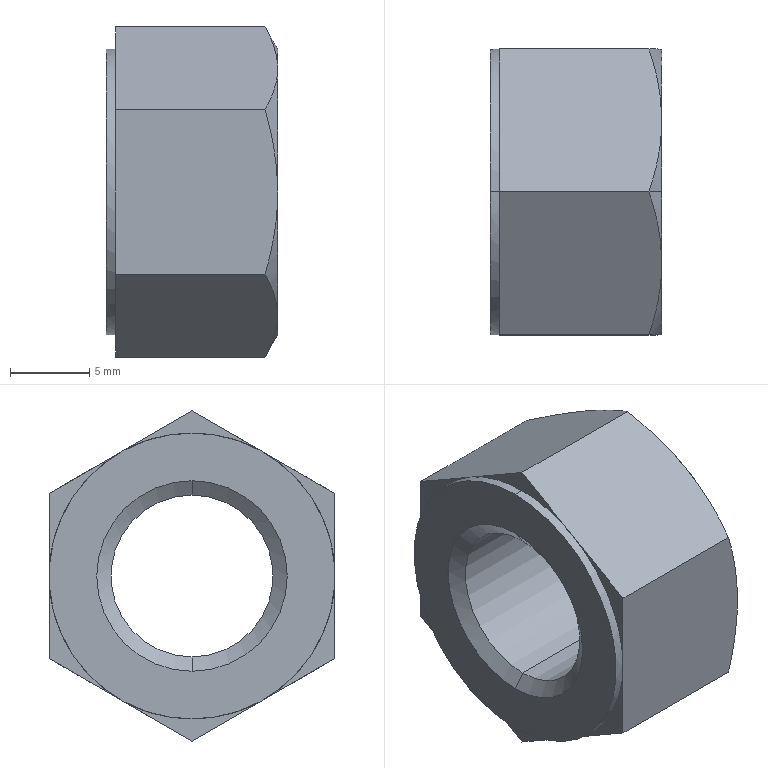Part | SolidWorks | features BaseBody 1 | 1 solid | 31 faces | box 10.8 x 18 x 20.785 mm | volume 2106 mm3 | plane 14 | cone 11 | cylinder 6 | commonest cylinder face diameters 10.2 x2 12 x2 18 x2
STEP:
#1=CARTESIAN_POINT('',(235.656,-84.,194.721));
#2=VERTEX_POINT('',#1);
#3=CARTESIAN_POINT('',(235.656,-84.,184.521));
#4=VERTEX_POINT('',#3);
#5=CARTESIAN_POINT('',(235.656,-84.,189.621));
#6=DIRECTION('',(1.,0.,0.));
#7=DIRECTION('',(0.,0.,-1.));
#8=AXIS2_PLACEMENT_3D('',#5,#6,#7);
#9=CIRCLE('',#8,5.1);
#10=EDGE_CURVE('',#2,#4,#9,.T.);
#11=ORIENTED_EDGE('',*,*,#10,.F.);
#12=CARTESIAN_POINT('',(245.17,-84.,194.721));
#13=VERTEX_POINT('',#12);
#14=CARTESIAN_POINT('',(235.,-84.,194.721));
#15=DIRECTION('',(1.,0.,0.));
#16=VECTOR('',#15,1000.);
#17=LINE('',#14,#16);
#18=EDGE_CURVE('',#2,#13,#17,.T.);
#19=ORIENTED_EDGE('',*,*,#18,.T.);
#20=CARTESIAN_POINT('',(245.17,-84.,184.521));
#21=VERTEX_POINT('',#20);
#22=CARTESIAN_POINT('',(245.17,-84.,189.621));
#23=DIRECTION('',(-1.,0.,0.));
#24=DIRECTION('',(0.,0.,-1.));
#25=AXIS2_PLACEMENT_3D('',#22,#23,#24);
#26=CIRCLE('',#25,5.1);
#27=EDGE_CURVE('',#21,#13,#26,.T.);
#28=ORIENTED_EDGE('',*,*,#27,.F.);
#29=CARTESIAN_POINT('',(235.,-84.,184.521));
#30=DIRECTION('',(1.,0.,0.));
#31=VECTOR('',#30,1000.);
#32=LINE('',#29,#31);
#33=EDGE_CURVE('',#4,#21,#32,.T.);
#34=ORIENTED_EDGE('',*,*,#33,.F.);
#35=EDGE_LOOP('',(#11,#19,#28,#34));
#36=FACE_OUTER_BOUND('',#35,.T.);
#37=CARTESIAN_POINT('',(235.,-84.,189.621));
#38=DIRECTION('',(1.,0.,0.));
#39=DIRECTION('',(0.,0.,-1.));
#40=AXIS2_PLACEMENT_3D('',#37,#38,#39);
#41=CYLINDRICAL_SURFACE('',#40,5.1);
#42=ADVANCED_FACE('',(#36),#41,.F.);
#43=ORIENTED_EDGE('',*,*,#27,.T.);
#44=CARTESIAN_POINT('',(245.8,-84.,195.621));
#45=VERTEX_POINT('',#44);
#46=CARTESIAN_POINT('',(245.8,-84.,195.621));
#47=DIRECTION('',(0.5736,0.,0.8192));
#48=VECTOR('',#47,1000.);
#49=LINE('',#46,#48);
#50=EDGE_CURVE('',#13,#45,#49,.T.);
#51=ORIENTED_EDGE('',*,*,#50,.T.);
#52=CARTESIAN_POINT('',(245.8,-84.,183.621));
#53=VERTEX_POINT('',#52);
#54=CARTESIAN_POINT('',(245.8,-84.,189.621));
#55=DIRECTION('',(-1.,0.,0.));
#56=DIRECTION('',(0.,0.,-1.));
#57=AXIS2_PLACEMENT_3D('',#54,#55,#56);
#58=CIRCLE('',#57,6.);
#59=EDGE_CURVE('',#53,#45,#58,.T.);
#60=ORIENTED_EDGE('',*,*,#59,.F.);
#61=CARTESIAN_POINT('',(245.8,-84.,183.621));
#62=DIRECTION('',(0.5736,0.,-0.8192));
#63=VECTOR('',#62,1000.);
#64=LINE('',#61,#63);
#65=EDGE_CURVE('',#21,#53,#64,.T.);
#66=ORIENTED_EDGE('',*,*,#65,.F.);
#67=EDGE_LOOP('',(#43,#51,#60,#66));
#68=FACE_OUTER_BOUND('',#67,.T.);
#69=CARTESIAN_POINT('',(245.8,-84.,189.621));
#70=DIRECTION('',(1.,0.,0.));
#71=DIRECTION('',(0.,0.,-1.));
#72=AXIS2_PLACEMENT_3D('',#69,#70,#71);
#73=CONICAL_SURFACE('',#72,6.,0.9599);
#74=ADVANCED_FACE('',(#68),#73,.F.);
#75=ORIENTED_EDGE('',*,*,#10,.T.);
#76=CARTESIAN_POINT('',(235.025,-84.,183.621));
#77=VERTEX_POINT('',#76);
#78=CARTESIAN_POINT('',(235.025,-84.,183.621));
#79=DIRECTION('',(-0.5736,0.,-0.8192));
#80=VECTOR('',#79,1000.);
#81=LINE('',#78,#80);
#82=EDGE_CURVE('',#4,#77,#81,.T.);
#83=ORIENTED_EDGE('',*,*,#82,.T.);
#84=CARTESIAN_POINT('',(235.025,-84.,195.621));
#85=VERTEX_POINT('',#84);
#86=CARTESIAN_POINT('',(235.025,-84.,189.621));
#87=DIRECTION('',(1.,0.,0.));
#88=DIRECTION('',(0.,-0.5,-0.866));
#89=AXIS2_PLACEMENT_3D('',#86,#87,#88);
#90=CIRCLE('',#89,6.);
#91=EDGE_CURVE('',#85,#77,#90,.T.);
#92=ORIENTED_EDGE('',*,*,#91,.F.);
#93=CARTESIAN_POINT('',(235.025,-84.,195.621));
#94=DIRECTION('',(-0.5736,0.,0.8192));
#95=VECTOR('',#94,1000.);
#96=LINE('',#93,#95);
#97=EDGE_CURVE('',#2,#85,#96,.T.);
#98=ORIENTED_EDGE('',*,*,#97,.F.);
#99=EDGE_LOOP('',(#75,#83,#92,#98));
#100=FACE_OUTER_BOUND('',#99,.T.);
#101=CARTESIAN_POINT('',(235.025,-84.,189.621));
#102=DIRECTION('',(-1.,0.,0.));
#103=DIRECTION('',(0.,0.,1.));
#104=AXIS2_PLACEMENT_3D('',#101,#102,#103);
#105=CONICAL_SURFACE('',#104,6.,0.9599);
#106=ADVANCED_FACE('',(#100),#105,.F.);
#107=CARTESIAN_POINT('',(235.,-84.,195.621));
#108=VERTEX_POINT('',#107);
#109=CARTESIAN_POINT('',(235.,-84.,183.621));
#110=VERTEX_POINT('',#109);
#111=CARTESIAN_POINT('',(235.,-84.,189.621));
#112=DIRECTION('',(1.,0.,0.));
#113=DIRECTION('',(0.,0.,-1.));
#114=AXIS2_PLACEMENT_3D('',#111,#112,#113);
#115=CIRCLE('',#114,6.);
#116=EDGE_CURVE('',#108,#110,#115,.T.);
#117=ORIENTED_EDGE('',*,*,#116,.F.);
#118=CARTESIAN_POINT('',(220.762,-84.,195.621));
#119=DIRECTION('',(1.,0.,0.));
#120=VECTOR('',#119,1000.);
#121=LINE('',#118,#120);
#122=EDGE_CURVE('',#108,#85,#121,.T.);
#123=ORIENTED_EDGE('',*,*,#122,.T.);
#124=ORIENTED_EDGE('',*,*,#91,.T.);
#125=CARTESIAN_POINT('',(220.762,-84.,183.621));
#126=DIRECTION('',(1.,0.,0.));
#127=VECTOR('',#126,1000.);
#128=LINE('',#125,#127);
#129=EDGE_CURVE('',#110,#77,#128,.T.);
#130=ORIENTED_EDGE('',*,*,#129,.F.);
#131=EDGE_LOOP('',(#117,#123,#124,#130));
#132=FACE_OUTER_BOUND('',#131,.T.);
#133=CARTESIAN_POINT('',(220.762,-84.,189.621));
#134=DIRECTION('',(1.,0.,0.));
#135=DIRECTION('',(0.,0.,-1.));
#136=AXIS2_PLACEMENT_3D('',#133,#134,#135);
#137=CYLINDRICAL_SURFACE('',#136,6.);
#138=ADVANCED_FACE('',(#132),#137,.F.);
#139=CARTESIAN_POINT('',(245.8,-88.5,197.415));
#140=VERTEX_POINT('',#139);
#141=CARTESIAN_POINT('',(245.8,-84.,198.621));
#142=VERTEX_POINT('',#141);
#143=CARTESIAN_POINT('',(245.8,-84.,189.621));
#144=DIRECTION('',(-1.,0.,0.));
#145=DIRECTION('',(0.,0.,1.));
#146=AXIS2_PLACEMENT_3D('',#143,#144,#145);
#147=CIRCLE('',#146,9.);
#148=EDGE_CURVE('',#140,#142,#147,.T.);
#149=ORIENTED_EDGE('',*,*,#148,.T.);
#150=CARTESIAN_POINT('',(244.996,-84.,200.013));
#151=VERTEX_POINT('',#150);
#152=CARTESIAN_POINT('',(244.991,-84.,200.022));
#153=DIRECTION('',(-0.5,0.,0.866));
#154=VECTOR('',#153,1000.);
#155=LINE('',#152,#154);
#156=EDGE_CURVE('',#142,#151,#155,.T.);
#157=ORIENTED_EDGE('',*,*,#156,.T.);
#158=CARTESIAN_POINT('',(244.996,-84.,200.013));
#159=CARTESIAN_POINT('',(245.241,-84.735,199.589));
#160=CARTESIAN_POINT('',(245.443,-85.476,199.161));
#161=CARTESIAN_POINT('',(245.723,-86.974,198.296));
#162=CARTESIAN_POINT('',(245.8,-87.732,197.859));
#163=CARTESIAN_POINT('',(245.8,-88.5,197.415));
#164=B_SPLINE_CURVE_WITH_KNOTS('',3,(#158,#159,#160,#161,#162,#163),.UNSPECIFIED.,.F.,.F.,(4,2,4),(0.,0.002629,0.005258),.UNSPECIFIED.);
#165=EDGE_CURVE('',#151,#140,#164,.T.);
#166=ORIENTED_EDGE('',*,*,#165,.T.);
#167=EDGE_LOOP('',(#149,#157,#166));
#168=FACE_OUTER_BOUND('',#167,.T.);
#169=CARTESIAN_POINT('',(244.991,-84.,189.621));
#170=DIRECTION('',(-1.,0.,0.));
#171=DIRECTION('',(0.,0.,1.));
#172=AXIS2_PLACEMENT_3D('',#169,#170,#171);
#173=CONICAL_SURFACE('',#172,10.401,1.047);
#174=ADVANCED_FACE('',(#168),#173,.T.);
#175=CARTESIAN_POINT('',(235.,-84.,198.621));
#176=VERTEX_POINT('',#175);
#177=CARTESIAN_POINT('',(235.,-84.,180.621));
#178=VERTEX_POINT('',#177);
#179=CARTESIAN_POINT('',(235.,-84.,189.621));
#180=DIRECTION('',(-1.,0.,0.));
#181=DIRECTION('',(0.,0.,-1.));
#182=AXIS2_PLACEMENT_3D('',#179,#180,#181);
#183=CIRCLE('',#182,9.);
#184=EDGE_CURVE('',#176,#178,#183,.T.);
#185=ORIENTED_EDGE('',*,*,#184,.F.);
#186=CARTESIAN_POINT('',(235.6,-84.,198.621));
#187=VERTEX_POINT('',#186);
#188=CARTESIAN_POINT('',(245.8,-84.,198.621));
#189=DIRECTION('',(1.,0.,0.));
#190=VECTOR('',#189,1000.);
#191=LINE('',#188,#190);
#192=EDGE_CURVE('',#176,#187,#191,.T.);
#193=ORIENTED_EDGE('',*,*,#192,.T.);
#194=CARTESIAN_POINT('',(235.6,-79.5,197.415));
#195=VERTEX_POINT('',#194);
#196=CARTESIAN_POINT('',(235.6,-84.,189.621));
#197=DIRECTION('',(-1.,0.,0.));
#198=DIRECTION('',(0.,0.,-1.));
#199=AXIS2_PLACEMENT_3D('',#196,#197,#198);
#200=CIRCLE('',#199,9.);
#201=EDGE_CURVE('',#187,#195,#200,.T.);
#202=ORIENTED_EDGE('',*,*,#201,.T.);
#203=CARTESIAN_POINT('',(235.6,-75.,189.621));
#204=VERTEX_POINT('',#203);
#205=CARTESIAN_POINT('',(235.6,-84.,189.621));
#206=DIRECTION('',(-1.,0.,0.));
#207=DIRECTION('',(0.,0.,-1.));
#208=AXIS2_PLACEMENT_3D('',#205,#206,#207);
#209=CIRCLE('',#208,9.);
#210=EDGE_CURVE('',#195,#204,#209,.T.);
#211=ORIENTED_EDGE('',*,*,#210,.T.);
#212=CARTESIAN_POINT('',(235.6,-79.5,181.827));
#213=VERTEX_POINT('',#212);
#214=CARTESIAN_POINT('',(235.6,-84.,189.621));
#215=DIRECTION('',(-1.,0.,0.));
#216=DIRECTION('',(0.,0.,-1.));
#217=AXIS2_PLACEMENT_3D('',#214,#215,#216);
#218=CIRCLE('',#217,9.);
#219=EDGE_CURVE('',#204,#213,#218,.T.);
#220=ORIENTED_EDGE('',*,*,#219,.T.);
#221=CARTESIAN_POINT('',(235.6,-84.,180.621));
#222=VERTEX_POINT('',#221);
#223=CARTESIAN_POINT('',(235.6,-84.,189.621));
#224=DIRECTION('',(-1.,0.,0.));
#225=DIRECTION('',(0.,0.,-1.));
#226=AXIS2_PLACEMENT_3D('',#223,#224,#225);
#227=CIRCLE('',#226,9.);
#228=EDGE_CURVE('',#213,#222,#227,.T.);
#229=ORIENTED_EDGE('',*,*,#228,.T.);
#230=CARTESIAN_POINT('',(245.8,-84.,180.621));
#231=DIRECTION('',(1.,0.,0.));
#232=VECTOR('',#231,1000.);
#233=LINE('',#230,#232);
#234=EDGE_CURVE('',#178,#222,#233,.T.);
#235=ORIENTED_EDGE('',*,*,#234,.F.);
#236=EDGE_LOOP('',(#185,#193,#202,#211,#220,#229,#235));
#237=FACE_OUTER_BOUND('',#236,.T.);
#238=CARTESIAN_POINT('',(245.8,-84.,189.621));
#239=DIRECTION('',(1.,0.,0.));
#240=DIRECTION('',(0.,0.,-1.));
#241=AXIS2_PLACEMENT_3D('',#238,#239,#240);
#242=CYLINDRICAL_SURFACE('',#241,9.);
#243=ADVANCED_FACE('',(#237),#242,.T.);
#244=ORIENTED_EDGE('',*,*,#18,.F.);
#245=CARTESIAN_POINT('',(235.656,-84.,189.621));
#246=DIRECTION('',(1.,0.,0.));
#247=DIRECTION('',(0.,0.,-1.));
#248=AXIS2_PLACEMENT_3D('',#245,#246,#247);
#249=CIRCLE('',#248,5.1);
#250=EDGE_CURVE('',#4,#2,#249,.T.);
#251=ORIENTED_EDGE('',*,*,#250,.F.);
#252=ORIENTED_EDGE('',*,*,#33,.T.);
#253=CARTESIAN_POINT('',(245.17,-84.,189.621));
#254=DIRECTION('',(-1.,0.,0.));
#255=DIRECTION('',(0.,0.,-1.));
#256=AXIS2_PLACEMENT_3D('',#253,#254,#255);
#257=CIRCLE('',#256,5.1);
#258=EDGE_CURVE('',#13,#21,#257,.T.);
#259=ORIENTED_EDGE('',*,*,#258,.F.);
#260=EDGE_LOOP('',(#244,#251,#252,#259));
#261=FACE_OUTER_BOUND('',#260,.T.);
#262=CARTESIAN_POINT('',(235.,-84.,189.621));
#263=DIRECTION('',(1.,0.,0.));
#264=DIRECTION('',(0.,0.,-1.));
#265=AXIS2_PLACEMENT_3D('',#262,#263,#264);
#266=CYLINDRICAL_SURFACE('',#265,5.1);
#267=ADVANCED_FACE('',(#261),#266,.F.);
#268=ORIENTED_EDGE('',*,*,#50,.F.);
#269=ORIENTED_EDGE('',*,*,#258,.T.);
#270=ORIENTED_EDGE('',*,*,#65,.T.);
#271=CARTESIAN_POINT('',(245.8,-84.,189.621));
#272=DIRECTION('',(-1.,0.,0.));
#273=DIRECTION('',(0.,0.,-1.));
#274=AXIS2_PLACEMENT_3D('',#271,#272,#273);
#275=CIRCLE('',#274,6.);
#276=EDGE_CURVE('',#45,#53,#275,.T.);
#277=ORIENTED_EDGE('',*,*,#276,.F.);
#278=EDGE_LOOP('',(#268,#269,#270,#277));
#279=FACE_OUTER_BOUND('',#278,.T.);
#280=CARTESIAN_POINT('',(245.8,-84.,189.621));
#281=DIRECTION('',(1.,0.,0.));
#282=DIRECTION('',(0.,0.,-1.));
#283=AXIS2_PLACEMENT_3D('',#280,#281,#282);
#284=CONICAL_SURFACE('',#283,6.,0.9599);
#285=ADVANCED_FACE('',(#279),#284,.F.);
#286=ORIENTED_EDGE('',*,*,#82,.F.);
#287=ORIENTED_EDGE('',*,*,#250,.T.);
#288=ORIENTED_EDGE('',*,*,#97,.T.);
#289=CARTESIAN_POINT('',(235.025,-84.,189.621));
#290=DIRECTION('',(1.,0.,0.));
#291=DIRECTION('',(0.,-0.5,-0.866));
#292=AXIS2_PLACEMENT_3D('',#289,#290,#291);
#293=CIRCLE('',#292,6.);
#294=EDGE_CURVE('',#77,#85,#293,.T.);
#295=ORIENTED_EDGE('',*,*,#294,.F.);
#296=EDGE_LOOP('',(#286,#287,#288,#295));
#297=FACE_OUTER_BOUND('',#296,.T.);
#298=CARTESIAN_POINT('',(235.025,-84.,189.621));
#299=DIRECTION('',(-1.,0.,0.));
#300=DIRECTION('',(0.,0.,1.));
#301=AXIS2_PLACEMENT_3D('',#298,#299,#300);
#302=CONICAL_SURFACE('',#301,6.,0.9599);
#303=ADVANCED_FACE('',(#297),#302,.F.);
#304=CARTESIAN_POINT('',(245.8,-79.5,181.827));
#305=VERTEX_POINT('',#304);
#306=CARTESIAN_POINT('',(245.8,-88.5,181.827));
#307=VERTEX_POINT('',#306);
#308=CARTESIAN_POINT('',(245.8,-84.,189.621));
#309=DIRECTION('',(-1.,0.,0.));
#310=DIRECTION('',(0.,0.,1.));
#311=AXIS2_PLACEMENT_3D('',#308,#309,#310);
#312=CIRCLE('',#311,9.);
#313=EDGE_CURVE('',#305,#307,#312,.T.);
#314=ORIENTED_EDGE('',*,*,#313,.F.);
#315=CARTESIAN_POINT('',(245.8,-75.,189.621));
#316=VERTEX_POINT('',#315);
#317=CARTESIAN_POINT('',(245.8,-84.,189.621));
#318=DIRECTION('',(-1.,0.,0.));
#319=DIRECTION('',(0.,0.,1.));
#320=AXIS2_PLACEMENT_3D('',#317,#318,#319);
#321=CIRCLE('',#320,9.);
#322=EDGE_CURVE('',#316,#305,#321,.T.);
#323=ORIENTED_EDGE('',*,*,#322,.F.);
#324=CARTESIAN_POINT('',(245.8,-79.5,197.415));
#325=VERTEX_POINT('',#324);
#326=CARTESIAN_POINT('',(245.8,-84.,189.621));
#327=DIRECTION('',(-1.,0.,0.));
#328=DIRECTION('',(0.,0.,1.));
#329=AXIS2_PLACEMENT_3D('',#326,#327,#328);
#330=CIRCLE('',#329,9.);
#331=EDGE_CURVE('',#325,#316,#330,.T.);
#332=ORIENTED_EDGE('',*,*,#331,.F.);
#333=CARTESIAN_POINT('',(245.8,-84.,189.621));
#334=DIRECTION('',(-1.,0.,0.));
#335=DIRECTION('',(0.,0.,1.));
#336=AXIS2_PLACEMENT_3D('',#333,#334,#335);
#337=CIRCLE('',#336,9.);
#338=EDGE_CURVE('',#142,#325,#337,.T.);
#339=ORIENTED_EDGE('',*,*,#338,.F.);
#340=ORIENTED_EDGE('',*,*,#148,.F.);
#341=CARTESIAN_POINT('',(245.8,-93.,189.621));
#342=VERTEX_POINT('',#341);
#343=CARTESIAN_POINT('',(245.8,-84.,189.621));
#344=DIRECTION('',(-1.,0.,0.));
#345=DIRECTION('',(0.,0.,1.));
#346=AXIS2_PLACEMENT_3D('',#343,#344,#345);
#347=CIRCLE('',#346,9.);
#348=EDGE_CURVE('',#342,#140,#347,.T.);
#349=ORIENTED_EDGE('',*,*,#348,.F.);
#350=CARTESIAN_POINT('',(245.8,-84.,189.621));
#351=DIRECTION('',(-1.,0.,0.));
#352=DIRECTION('',(0.,0.,1.));
#353=AXIS2_PLACEMENT_3D('',#350,#351,#352);
#354=CIRCLE('',#353,9.);
#355=EDGE_CURVE('',#307,#342,#354,.T.);
#356=ORIENTED_EDGE('',*,*,#355,.F.);
#357=EDGE_LOOP('',(#314,#323,#332,#339,#340,#349,#356));
#358=FACE_OUTER_BOUND('',#357,.T.);
#359=ORIENTED_EDGE('',*,*,#59,.T.);
#360=ORIENTED_EDGE('',*,*,#276,.T.);
#361=EDGE_LOOP('',(#359,#360));
#362=FACE_BOUND('',#361,.T.);
#363=CARTESIAN_POINT('',(245.8,-93.,194.817));
#364=DIRECTION('',(-1.,0.,0.));
#365=DIRECTION('',(0.,0.,1.));
#366=AXIS2_PLACEMENT_3D('',#363,#364,#365);
#367=PLANE('',#366);
#368=ADVANCED_FACE('',(#358,#362),#367,.F.);
#369=ORIENTED_EDGE('',*,*,#122,.F.);
#370=CARTESIAN_POINT('',(235.,-84.,189.621));
#371=DIRECTION('',(1.,0.,0.));
#372=DIRECTION('',(0.,0.,-1.));
#373=AXIS2_PLACEMENT_3D('',#370,#371,#372);
#374=CIRCLE('',#373,6.);
#375=EDGE_CURVE('',#110,#108,#374,.T.);
#376=ORIENTED_EDGE('',*,*,#375,.F.);
#377=ORIENTED_EDGE('',*,*,#129,.T.);
#378=ORIENTED_EDGE('',*,*,#294,.T.);
#379=EDGE_LOOP('',(#369,#376,#377,#378));
#380=FACE_OUTER_BOUND('',#379,.T.);
#381=CARTESIAN_POINT('',(220.762,-84.,189.621));
#382=DIRECTION('',(1.,0.,0.));
#383=DIRECTION('',(0.,0.,-1.));
#384=AXIS2_PLACEMENT_3D('',#381,#382,#383);
#385=CYLINDRICAL_SURFACE('',#384,6.);
#386=ADVANCED_FACE('',(#380),#385,.F.);
#387=ORIENTED_EDGE('',*,*,#355,.T.);
#388=CARTESIAN_POINT('',(244.996,-93.,184.425));
#389=VERTEX_POINT('',#388);
#390=CARTESIAN_POINT('',(245.8,-93.,189.621));
#391=CARTESIAN_POINT('',(245.8,-93.,188.734));
#392=CARTESIAN_POINT('',(245.723,-93.,187.859));
#393=CARTESIAN_POINT('',(245.443,-93.,186.129));
#394=CARTESIAN_POINT('',(245.241,-93.,185.274));
#395=CARTESIAN_POINT('',(244.996,-93.,184.425));
#396=B_SPLINE_CURVE_WITH_KNOTS('',3,(#390,#391,#392,#393,#394,#395),.UNSPECIFIED.,.F.,.F.,(4,2,4),(0.,0.002629,0.005258),.UNSPECIFIED.);
#397=EDGE_CURVE('',#342,#389,#396,.T.);
#398=ORIENTED_EDGE('',*,*,#397,.T.);
#399=CARTESIAN_POINT('',(244.996,-93.,184.425));
#400=CARTESIAN_POINT('',(245.241,-92.265,184.001));
#401=CARTESIAN_POINT('',(245.443,-91.524,183.573));
#402=CARTESIAN_POINT('',(245.723,-90.026,182.708));
#403=CARTESIAN_POINT('',(245.8,-89.268,182.27));
#404=CARTESIAN_POINT('',(245.8,-88.5,181.827));
#405=B_SPLINE_CURVE_WITH_KNOTS('',3,(#399,#400,#401,#402,#403,#404),.UNSPECIFIED.,.F.,.F.,(4,2,4),(0.,0.002629,0.005258),.UNSPECIFIED.);
#406=EDGE_CURVE('',#389,#307,#405,.T.);
#407=ORIENTED_EDGE('',*,*,#406,.T.);
#408=EDGE_LOOP('',(#387,#398,#407));
#409=FACE_OUTER_BOUND('',#408,.T.);
#410=CARTESIAN_POINT('',(244.991,-84.,189.621));
#411=DIRECTION('',(-1.,0.,0.));
#412=DIRECTION('',(0.,0.,1.));
#413=AXIS2_PLACEMENT_3D('',#410,#411,#412);
#414=CONICAL_SURFACE('',#413,10.401,1.047);
#415=ADVANCED_FACE('',(#409),#414,.T.);
#416=CARTESIAN_POINT('',(244.996,-84.,179.229));
#417=VERTEX_POINT('',#416);
#418=CARTESIAN_POINT('',(245.8,-88.5,181.827));
#419=CARTESIAN_POINT('',(245.8,-87.732,181.383));
#420=CARTESIAN_POINT('',(245.723,-86.974,180.946));
#421=CARTESIAN_POINT('',(245.443,-85.476,180.081));
#422=CARTESIAN_POINT('',(245.241,-84.735,179.653));
#423=CARTESIAN_POINT('',(244.996,-84.,179.229));
#424=B_SPLINE_CURVE_WITH_KNOTS('',3,(#418,#419,#420,#421,#422,#423),.UNSPECIFIED.,.F.,.F.,(4,2,4),(0.,0.002629,0.005258),.UNSPECIFIED.);
#425=EDGE_CURVE('',#307,#417,#424,.T.);
#426=ORIENTED_EDGE('',*,*,#425,.T.);
#427=CARTESIAN_POINT('',(244.996,-84.,179.229));
#428=CARTESIAN_POINT('',(245.241,-83.265,179.653));
#429=CARTESIAN_POINT('',(245.443,-82.524,180.081));
#430=CARTESIAN_POINT('',(245.723,-81.026,180.946));
#431=CARTESIAN_POINT('',(245.8,-80.268,181.383));
#432=CARTESIAN_POINT('',(245.8,-79.5,181.827));
#433=B_SPLINE_CURVE_WITH_KNOTS('',3,(#427,#428,#429,#430,#431,#432),.UNSPECIFIED.,.F.,.F.,(4,2,4),(0.,0.002629,0.005258),.UNSPECIFIED.);
#434=EDGE_CURVE('',#417,#305,#433,.T.);
#435=ORIENTED_EDGE('',*,*,#434,.T.);
#436=ORIENTED_EDGE('',*,*,#313,.T.);
#437=EDGE_LOOP('',(#426,#435,#436));
#438=FACE_OUTER_BOUND('',#437,.T.);
#439=CARTESIAN_POINT('',(244.991,-84.,189.621));
#440=DIRECTION('',(-1.,0.,0.));
#441=DIRECTION('',(0.,0.,1.));
#442=AXIS2_PLACEMENT_3D('',#439,#440,#441);
#443=CONICAL_SURFACE('',#442,10.401,1.047);
#444=ADVANCED_FACE('',(#438),#443,.T.);
#445=CARTESIAN_POINT('',(244.996,-75.,184.425));
#446=VERTEX_POINT('',#445);
#447=CARTESIAN_POINT('',(245.8,-79.5,181.827));
#448=CARTESIAN_POINT('',(245.8,-78.732,182.27));
#449=CARTESIAN_POINT('',(245.723,-77.974,182.708));
#450=CARTESIAN_POINT('',(245.443,-76.476,183.573));
#451=CARTESIAN_POINT('',(245.241,-75.735,184.001));
#452=CARTESIAN_POINT('',(244.996,-75.,184.425));
#453=B_SPLINE_CURVE_WITH_KNOTS('',3,(#447,#448,#449,#450,#451,#452),.UNSPECIFIED.,.F.,.F.,(4,2,4),(0.,0.002629,0.005258),.UNSPECIFIED.);
#454=EDGE_CURVE('',#305,#446,#453,.T.);
#455=ORIENTED_EDGE('',*,*,#454,.T.);
#456=CARTESIAN_POINT('',(244.996,-75.,184.425));
#457=CARTESIAN_POINT('',(245.241,-75.,185.274));
#458=CARTESIAN_POINT('',(245.443,-75.,186.129));
#459=CARTESIAN_POINT('',(245.723,-75.,187.859));
#460=CARTESIAN_POINT('',(245.8,-75.,188.734));
#461=CARTESIAN_POINT('',(245.8,-75.,189.621));
#462=B_SPLINE_CURVE_WITH_KNOTS('',3,(#456,#457,#458,#459,#460,#461),.UNSPECIFIED.,.F.,.F.,(4,2,4),(0.,0.002629,0.005258),.UNSPECIFIED.);
#463=EDGE_CURVE('',#446,#316,#462,.T.);
#464=ORIENTED_EDGE('',*,*,#463,.T.);
#465=ORIENTED_EDGE('',*,*,#322,.T.);
#466=EDGE_LOOP('',(#455,#464,#465));
#467=FACE_OUTER_BOUND('',#466,.T.);
#468=CARTESIAN_POINT('',(244.991,-84.,189.621));
#469=DIRECTION('',(-1.,0.,0.));
#470=DIRECTION('',(0.,0.,1.));
#471=AXIS2_PLACEMENT_3D('',#468,#469,#470);
#472=CONICAL_SURFACE('',#471,10.401,1.047);
#473=ADVANCED_FACE('',(#467),#472,.T.);
#474=ORIENTED_EDGE('',*,*,#331,.T.);
#475=CARTESIAN_POINT('',(244.996,-75.,194.817));
#476=VERTEX_POINT('',#475);
#477=CARTESIAN_POINT('',(245.8,-75.,189.621));
#478=CARTESIAN_POINT('',(245.8,-75.,190.508));
#479=CARTESIAN_POINT('',(245.723,-75.,191.383));
#480=CARTESIAN_POINT('',(245.443,-75.,193.113));
#481=CARTESIAN_POINT('',(245.241,-75.,193.968));
#482=CARTESIAN_POINT('',(244.996,-75.,194.817));
#483=B_SPLINE_CURVE_WITH_KNOTS('',3,(#477,#478,#479,#480,#481,#482),.UNSPECIFIED.,.F.,.F.,(4,2,4),(0.,0.002629,0.005258),.UNSPECIFIED.);
#484=EDGE_CURVE('',#316,#476,#483,.T.);
#485=ORIENTED_EDGE('',*,*,#484,.T.);
#486=CARTESIAN_POINT('',(244.996,-75.,194.817));
#487=CARTESIAN_POINT('',(245.241,-75.735,195.242));
#488=CARTESIAN_POINT('',(245.443,-76.476,195.669));
#489=CARTESIAN_POINT('',(245.723,-77.974,196.535));
#490=CARTESIAN_POINT('',(245.8,-78.732,196.972));
#491=CARTESIAN_POINT('',(245.8,-79.5,197.415));
#492=B_SPLINE_CURVE_WITH_KNOTS('',3,(#486,#487,#488,#489,#490,#491),.UNSPECIFIED.,.F.,.F.,(4,2,4),(0.,0.002629,0.005258),.UNSPECIFIED.);
#493=EDGE_CURVE('',#476,#325,#492,.T.);
#494=ORIENTED_EDGE('',*,*,#493,.T.);
#495=EDGE_LOOP('',(#474,#485,#494));
#496=FACE_OUTER_BOUND('',#495,.T.);
#497=CARTESIAN_POINT('',(244.991,-84.,189.621));
#498=DIRECTION('',(-1.,0.,0.));
#499=DIRECTION('',(0.,0.,1.));
#500=AXIS2_PLACEMENT_3D('',#497,#498,#499);
#501=CONICAL_SURFACE('',#500,10.401,1.047);
#502=ADVANCED_FACE('',(#496),#501,.T.);
#503=ORIENTED_EDGE('',*,*,#156,.F.);
#504=ORIENTED_EDGE('',*,*,#338,.T.);
#505=CARTESIAN_POINT('',(245.8,-79.5,197.415));
#506=CARTESIAN_POINT('',(245.8,-80.268,197.859));
#507=CARTESIAN_POINT('',(245.723,-81.026,198.296));
#508=CARTESIAN_POINT('',(245.443,-82.524,199.161));
#509=CARTESIAN_POINT('',(245.241,-83.265,199.589));
#510=CARTESIAN_POINT('',(244.996,-84.,200.013));
#511=B_SPLINE_CURVE_WITH_KNOTS('',3,(#505,#506,#507,#508,#509,#510),.UNSPECIFIED.,.F.,.F.,(4,2,4),(0.,0.002629,0.005258),.UNSPECIFIED.);
#512=EDGE_CURVE('',#325,#151,#511,.T.);
#513=ORIENTED_EDGE('',*,*,#512,.T.);
#514=EDGE_LOOP('',(#503,#504,#513));
#515=FACE_OUTER_BOUND('',#514,.T.);
#516=CARTESIAN_POINT('',(244.991,-84.,189.621));
#517=DIRECTION('',(-1.,0.,0.));
#518=DIRECTION('',(0.,0.,1.));
#519=AXIS2_PLACEMENT_3D('',#516,#517,#518);
#520=CONICAL_SURFACE('',#519,10.401,1.047);
#521=ADVANCED_FACE('',(#515),#520,.T.);
#522=CARTESIAN_POINT('',(244.996,-93.,194.817));
#523=VERTEX_POINT('',#522);
#524=CARTESIAN_POINT('',(245.8,-88.5,197.415));
#525=CARTESIAN_POINT('',(245.8,-89.268,196.972));
#526=CARTESIAN_POINT('',(245.723,-90.026,196.535));
#527=CARTESIAN_POINT('',(245.443,-91.524,195.669));
#528=CARTESIAN_POINT('',(245.241,-92.265,195.242));
#529=CARTESIAN_POINT('',(244.996,-93.,194.817));
#530=B_SPLINE_CURVE_WITH_KNOTS('',3,(#524,#525,#526,#527,#528,#529),.UNSPECIFIED.,.F.,.F.,(4,2,4),(0.,0.002629,0.005258),.UNSPECIFIED.);
#531=EDGE_CURVE('',#140,#523,#530,.T.);
#532=ORIENTED_EDGE('',*,*,#531,.T.);
#533=CARTESIAN_POINT('',(244.996,-93.,194.817));
#534=CARTESIAN_POINT('',(245.241,-93.,193.968));
#535=CARTESIAN_POINT('',(245.443,-93.,193.113));
#536=CARTESIAN_POINT('',(245.723,-93.,191.383));
#537=CARTESIAN_POINT('',(245.8,-93.,190.508));
#538=CARTESIAN_POINT('',(245.8,-93.,189.621));
#539=B_SPLINE_CURVE_WITH_KNOTS('',3,(#533,#534,#535,#536,#537,#538),.UNSPECIFIED.,.F.,.F.,(4,2,4),(0.,0.002629,0.005258),.UNSPECIFIED.);
#540=EDGE_CURVE('',#523,#342,#539,.T.);
#541=ORIENTED_EDGE('',*,*,#540,.T.);
#542=ORIENTED_EDGE('',*,*,#348,.T.);
#543=EDGE_LOOP('',(#532,#541,#542));
#544=FACE_OUTER_BOUND('',#543,.T.);
#545=CARTESIAN_POINT('',(244.991,-84.,189.621));
#546=DIRECTION('',(-1.,0.,0.));
#547=DIRECTION('',(0.,0.,1.));
#548=AXIS2_PLACEMENT_3D('',#545,#546,#547);
#549=CONICAL_SURFACE('',#548,10.401,1.047);
#550=ADVANCED_FACE('',(#544),#549,.T.);
#551=CARTESIAN_POINT('',(235.,-84.,189.621));
#552=DIRECTION('',(-1.,0.,0.));
#553=DIRECTION('',(0.,0.,-1.));
#554=AXIS2_PLACEMENT_3D('',#551,#552,#553);
#555=CIRCLE('',#554,9.);
#556=EDGE_CURVE('',#178,#176,#555,.T.);
#557=ORIENTED_EDGE('',*,*,#556,.T.);
#558=ORIENTED_EDGE('',*,*,#184,.T.);
#559=EDGE_LOOP('',(#557,#558));
#560=FACE_OUTER_BOUND('',#559,.T.);
#561=ORIENTED_EDGE('',*,*,#375,.T.);
#562=ORIENTED_EDGE('',*,*,#116,.T.);
#563=EDGE_LOOP('',(#561,#562));
#564=FACE_BOUND('',#563,.T.);
#565=CARTESIAN_POINT('',(235.,-93.,194.817));
#566=DIRECTION('',(-1.,0.,0.));
#567=DIRECTION('',(0.,0.,1.));
#568=AXIS2_PLACEMENT_3D('',#565,#566,#567);
#569=PLANE('',#568);
#570=ADVANCED_FACE('',(#560,#564),#569,.T.);
#571=CARTESIAN_POINT('',(235.6,-93.,194.817));
#572=VERTEX_POINT('',#571);
#573=CARTESIAN_POINT('',(235.6,-93.,189.621));
#574=VERTEX_POINT('',#573);
#575=CARTESIAN_POINT('',(235.6,-93.,194.817));
#576=DIRECTION('',(0.,0.,-1.));
#577=VECTOR('',#576,1000.);
#578=LINE('',#575,#577);
#579=EDGE_CURVE('',#572,#574,#578,.T.);
#580=ORIENTED_EDGE('',*,*,#579,.T.);
#581=CARTESIAN_POINT('',(235.6,-93.,184.425));
#582=VERTEX_POINT('',#581);
#583=CARTESIAN_POINT('',(235.6,-93.,194.817));
#584=DIRECTION('',(0.,0.,-1.));
#585=VECTOR('',#584,1000.);
#586=LINE('',#583,#585);
#587=EDGE_CURVE('',#574,#582,#586,.T.);
#588=ORIENTED_EDGE('',*,*,#587,.T.);
#589=CARTESIAN_POINT('',(235.,-93.,184.425));
#590=DIRECTION('',(1.,0.,0.));
#591=VECTOR('',#590,1000.);
#592=LINE('',#589,#591);
#593=EDGE_CURVE('',#582,#389,#592,.T.);
#594=ORIENTED_EDGE('',*,*,#593,.T.);
#595=ORIENTED_EDGE('',*,*,#397,.F.);
#596=ORIENTED_EDGE('',*,*,#540,.F.);
#597=CARTESIAN_POINT('',(235.,-93.,194.817));
#598=DIRECTION('',(-1.,0.,0.));
#599=VECTOR('',#598,1000.);
#600=LINE('',#597,#599);
#601=EDGE_CURVE('',#523,#572,#600,.T.);
#602=ORIENTED_EDGE('',*,*,#601,.T.);
#603=EDGE_LOOP('',(#580,#588,#594,#595,#596,#602));
#604=FACE_OUTER_BOUND('',#603,.T.);
#605=CARTESIAN_POINT('',(235.,-93.,194.817));
#606=DIRECTION('',(0.,-1.,0.));
#607=DIRECTION('',(0.,0.,-1.));
#608=AXIS2_PLACEMENT_3D('',#605,#606,#607);
#609=PLANE('',#608);
#610=ADVANCED_FACE('',(#604),#609,.T.);
#611=CARTESIAN_POINT('',(235.6,-88.5,181.827));
#612=VERTEX_POINT('',#611);
#613=CARTESIAN_POINT('',(235.6,-93.,184.425));
#614=DIRECTION('',(0.,0.866,-0.5));
#615=VECTOR('',#614,1000.);
#616=LINE('',#613,#615);
#617=EDGE_CURVE('',#582,#612,#616,.T.);
#618=ORIENTED_EDGE('',*,*,#617,.T.);
#619=CARTESIAN_POINT('',(235.6,-84.,179.229));
#620=VERTEX_POINT('',#619);
#621=CARTESIAN_POINT('',(235.6,-93.,184.425));
#622=DIRECTION('',(0.,0.866,-0.5));
#623=VECTOR('',#622,1000.);
#624=LINE('',#621,#623);
#625=EDGE_CURVE('',#612,#620,#624,.T.);
#626=ORIENTED_EDGE('',*,*,#625,.T.);
#627=CARTESIAN_POINT('',(235.,-84.,179.229));
#628=DIRECTION('',(1.,0.,0.));
#629=VECTOR('',#628,1000.);
#630=LINE('',#627,#629);
#631=EDGE_CURVE('',#620,#417,#630,.T.);
#632=ORIENTED_EDGE('',*,*,#631,.T.);
#633=ORIENTED_EDGE('',*,*,#425,.F.);
#634=ORIENTED_EDGE('',*,*,#406,.F.);
#635=ORIENTED_EDGE('',*,*,#593,.F.);
#636=EDGE_LOOP('',(#618,#626,#632,#633,#634,#635));
#637=FACE_OUTER_BOUND('',#636,.T.);
#638=CARTESIAN_POINT('',(235.,-93.,184.425));
#639=DIRECTION('',(0.,-0.5,-0.866));
#640=DIRECTION('',(0.,0.866,-0.5));
#641=AXIS2_PLACEMENT_3D('',#638,#639,#640);
#642=PLANE('',#641);
#643=ADVANCED_FACE('',(#637),#642,.T.);
#644=CARTESIAN_POINT('',(235.6,-84.,179.229));
#645=DIRECTION('',(0.,0.866,0.5));
#646=VECTOR('',#645,1000.);
#647=LINE('',#644,#646);
#648=EDGE_CURVE('',#620,#213,#647,.T.);
#649=ORIENTED_EDGE('',*,*,#648,.T.);
#650=CARTESIAN_POINT('',(235.6,-75.,184.425));
#651=VERTEX_POINT('',#650);
#652=CARTESIAN_POINT('',(235.6,-84.,179.229));
#653=DIRECTION('',(0.,0.866,0.5));
#654=VECTOR('',#653,1000.);
#655=LINE('',#652,#654);
#656=EDGE_CURVE('',#213,#651,#655,.T.);
#657=ORIENTED_EDGE('',*,*,#656,.T.);
#658=CARTESIAN_POINT('',(235.,-75.,184.425));
#659=DIRECTION('',(1.,0.,0.));
#660=VECTOR('',#659,1000.);
#661=LINE('',#658,#660);
#662=EDGE_CURVE('',#651,#446,#661,.T.);
#663=ORIENTED_EDGE('',*,*,#662,.T.);
#664=ORIENTED_EDGE('',*,*,#454,.F.);
#665=ORIENTED_EDGE('',*,*,#434,.F.);
#666=ORIENTED_EDGE('',*,*,#631,.F.);
#667=EDGE_LOOP('',(#649,#657,#663,#664,#665,#666));
#668=FACE_OUTER_BOUND('',#667,.T.);
#669=CARTESIAN_POINT('',(235.,-84.,179.229));
#670=DIRECTION('',(0.,0.5,-0.866));
#671=DIRECTION('',(0.,0.866,0.5));
#672=AXIS2_PLACEMENT_3D('',#669,#670,#671);
#673=PLANE('',#672);
#674=ADVANCED_FACE('',(#668),#673,.T.);
#675=CARTESIAN_POINT('',(235.6,-75.,184.425));
#676=DIRECTION('',(0.,0.,1.));
#677=VECTOR('',#676,1000.);
#678=LINE('',#675,#677);
#679=EDGE_CURVE('',#651,#204,#678,.T.);
#680=ORIENTED_EDGE('',*,*,#679,.T.);
#681=CARTESIAN_POINT('',(235.6,-75.,194.817));
#682=VERTEX_POINT('',#681);
#683=CARTESIAN_POINT('',(235.6,-75.,184.425));
#684=DIRECTION('',(0.,0.,1.));
#685=VECTOR('',#684,1000.);
#686=LINE('',#683,#685);
#687=EDGE_CURVE('',#204,#682,#686,.T.);
#688=ORIENTED_EDGE('',*,*,#687,.T.);
#689=CARTESIAN_POINT('',(235.,-75.,194.817));
#690=DIRECTION('',(1.,0.,0.));
#691=VECTOR('',#690,1000.);
#692=LINE('',#689,#691);
#693=EDGE_CURVE('',#682,#476,#692,.T.);
#694=ORIENTED_EDGE('',*,*,#693,.T.);
#695=ORIENTED_EDGE('',*,*,#484,.F.);
#696=ORIENTED_EDGE('',*,*,#463,.F.);
#697=ORIENTED_EDGE('',*,*,#662,.F.);
#698=EDGE_LOOP('',(#680,#688,#694,#695,#696,#697));
#699=FACE_OUTER_BOUND('',#698,.T.);
#700=CARTESIAN_POINT('',(235.,-75.,184.425));
#701=DIRECTION('',(0.,1.,0.));
#702=DIRECTION('',(0.,0.,1.));
#703=AXIS2_PLACEMENT_3D('',#700,#701,#702);
#704=PLANE('',#703);
#705=ADVANCED_FACE('',(#699),#704,.T.);
#706=ORIENTED_EDGE('',*,*,#693,.F.);
#707=CARTESIAN_POINT('',(235.6,-84.,200.013));
#708=DIRECTION('',(0.,0.866,-0.5));
#709=VECTOR('',#708,1000.);
#710=LINE('',#707,#709);
#711=EDGE_CURVE('',#195,#682,#710,.T.);
#712=ORIENTED_EDGE('',*,*,#711,.F.);
#713=CARTESIAN_POINT('',(235.6,-84.,200.013));
#714=VERTEX_POINT('',#713);
#715=CARTESIAN_POINT('',(235.6,-84.,200.013));
#716=DIRECTION('',(0.,0.866,-0.5));
#717=VECTOR('',#716,1000.);
#718=LINE('',#715,#717);
#719=EDGE_CURVE('',#714,#195,#718,.T.);
#720=ORIENTED_EDGE('',*,*,#719,.F.);
#721=CARTESIAN_POINT('',(235.,-84.,200.013));
#722=DIRECTION('',(-1.,0.,0.));
#723=VECTOR('',#722,1000.);
#724=LINE('',#721,#723);
#725=EDGE_CURVE('',#151,#714,#724,.T.);
#726=ORIENTED_EDGE('',*,*,#725,.F.);
#727=ORIENTED_EDGE('',*,*,#512,.F.);
#728=ORIENTED_EDGE('',*,*,#493,.F.);
#729=EDGE_LOOP('',(#706,#712,#720,#726,#727,#728));
#730=FACE_OUTER_BOUND('',#729,.T.);
#731=CARTESIAN_POINT('',(235.,-84.,200.013));
#732=DIRECTION('',(0.,-0.5,-0.866));
#733=DIRECTION('',(0.,0.866,-0.5));
#734=AXIS2_PLACEMENT_3D('',#731,#732,#733);
#735=PLANE('',#734);
#736=ADVANCED_FACE('',(#730),#735,.F.);
#737=CARTESIAN_POINT('',(235.6,-88.5,197.415));
#738=VERTEX_POINT('',#737);
#739=CARTESIAN_POINT('',(235.6,-84.,200.013));
#740=DIRECTION('',(0.,-0.866,-0.5));
#741=VECTOR('',#740,1000.);
#742=LINE('',#739,#741);
#743=EDGE_CURVE('',#714,#738,#742,.T.);
#744=ORIENTED_EDGE('',*,*,#743,.T.);
#745=CARTESIAN_POINT('',(235.6,-84.,200.013));
#746=DIRECTION('',(0.,-0.866,-0.5));
#747=VECTOR('',#746,1000.);
#748=LINE('',#745,#747);
#749=EDGE_CURVE('',#738,#572,#748,.T.);
#750=ORIENTED_EDGE('',*,*,#749,.T.);
#751=ORIENTED_EDGE('',*,*,#601,.F.);
#752=ORIENTED_EDGE('',*,*,#531,.F.);
#753=ORIENTED_EDGE('',*,*,#165,.F.);
#754=ORIENTED_EDGE('',*,*,#725,.T.);
#755=EDGE_LOOP('',(#744,#750,#751,#752,#753,#754));
#756=FACE_OUTER_BOUND('',#755,.T.);
#757=CARTESIAN_POINT('',(235.,-84.,200.013));
#758=DIRECTION('',(0.,-0.5,0.866));
#759=DIRECTION('',(0.,-0.866,-0.5));
#760=AXIS2_PLACEMENT_3D('',#757,#758,#759);
#761=PLANE('',#760);
#762=ADVANCED_FACE('',(#756),#761,.T.);
#763=ORIENTED_EDGE('',*,*,#192,.F.);
#764=ORIENTED_EDGE('',*,*,#556,.F.);
#765=ORIENTED_EDGE('',*,*,#234,.T.);
#766=CARTESIAN_POINT('',(235.6,-84.,189.621));
#767=DIRECTION('',(-1.,0.,0.));
#768=DIRECTION('',(0.,0.,-1.));
#769=AXIS2_PLACEMENT_3D('',#766,#767,#768);
#770=CIRCLE('',#769,9.);
#771=EDGE_CURVE('',#222,#612,#770,.T.);
#772=ORIENTED_EDGE('',*,*,#771,.T.);
#773=CARTESIAN_POINT('',(235.6,-84.,189.621));
#774=DIRECTION('',(-1.,0.,0.));
#775=DIRECTION('',(0.,0.,-1.));
#776=AXIS2_PLACEMENT_3D('',#773,#774,#775);
#777=CIRCLE('',#776,9.);
#778=EDGE_CURVE('',#612,#574,#777,.T.);
#779=ORIENTED_EDGE('',*,*,#778,.T.);
#780=CARTESIAN_POINT('',(235.6,-84.,189.621));
#781=DIRECTION('',(-1.,0.,0.));
#782=DIRECTION('',(0.,0.,-1.));
#783=AXIS2_PLACEMENT_3D('',#780,#781,#782);
#784=CIRCLE('',#783,9.);
#785=EDGE_CURVE('',#574,#738,#784,.T.);
#786=ORIENTED_EDGE('',*,*,#785,.T.);
#787=CARTESIAN_POINT('',(235.6,-84.,189.621));
#788=DIRECTION('',(-1.,0.,0.));
#789=DIRECTION('',(0.,0.,-1.));
#790=AXIS2_PLACEMENT_3D('',#787,#788,#789);
#791=CIRCLE('',#790,9.);
#792=EDGE_CURVE('',#738,#187,#791,.T.);
#793=ORIENTED_EDGE('',*,*,#792,.T.);
#794=EDGE_LOOP('',(#763,#764,#765,#772,#779,#786,#793));
#795=FACE_OUTER_BOUND('',#794,.T.);
#796=CARTESIAN_POINT('',(245.8,-84.,189.621));
#797=DIRECTION('',(1.,0.,0.));
#798=DIRECTION('',(0.,0.,-1.));
#799=AXIS2_PLACEMENT_3D('',#796,#797,#798);
#800=CYLINDRICAL_SURFACE('',#799,9.);
#801=ADVANCED_FACE('',(#795),#800,.T.);
#802=ORIENTED_EDGE('',*,*,#617,.F.);
#803=ORIENTED_EDGE('',*,*,#587,.F.);
#804=ORIENTED_EDGE('',*,*,#778,.F.);
#805=EDGE_LOOP('',(#802,#803,#804));
#806=FACE_OUTER_BOUND('',#805,.T.);
#807=CARTESIAN_POINT('',(235.6,-101.66,199.817));
#808=DIRECTION('',(-1.,0.,0.));
#809=DIRECTION('',(0.,0.,1.));
#810=AXIS2_PLACEMENT_3D('',#807,#808,#809);
#811=PLANE('',#810);
#812=ADVANCED_FACE('',(#806),#811,.T.);
#813=ORIENTED_EDGE('',*,*,#579,.F.);
#814=ORIENTED_EDGE('',*,*,#749,.F.);
#815=ORIENTED_EDGE('',*,*,#785,.F.);
#816=EDGE_LOOP('',(#813,#814,#815));
#817=FACE_OUTER_BOUND('',#816,.T.);
#818=CARTESIAN_POINT('',(235.6,-101.66,199.817));
#819=DIRECTION('',(-1.,0.,0.));
#820=DIRECTION('',(0.,0.,1.));
#821=AXIS2_PLACEMENT_3D('',#818,#819,#820);
#822=PLANE('',#821);
#823=ADVANCED_FACE('',(#817),#822,.T.);
#824=ORIENTED_EDGE('',*,*,#228,.F.);
#825=ORIENTED_EDGE('',*,*,#648,.F.);
#826=ORIENTED_EDGE('',*,*,#625,.F.);
#827=ORIENTED_EDGE('',*,*,#771,.F.);
#828=EDGE_LOOP('',(#824,#825,#826,#827));
#829=FACE_OUTER_BOUND('',#828,.T.);
#830=CARTESIAN_POINT('',(235.6,-101.66,199.817));
#831=DIRECTION('',(-1.,0.,0.));
#832=DIRECTION('',(0.,0.,1.));
#833=AXIS2_PLACEMENT_3D('',#830,#831,#832);
#834=PLANE('',#833);
#835=ADVANCED_FACE('',(#829),#834,.T.);
#836=ORIENTED_EDGE('',*,*,#219,.F.);
#837=ORIENTED_EDGE('',*,*,#679,.F.);
#838=ORIENTED_EDGE('',*,*,#656,.F.);
#839=EDGE_LOOP('',(#836,#837,#838));
#840=FACE_OUTER_BOUND('',#839,.T.);
#841=CARTESIAN_POINT('',(235.6,-101.66,199.817));
#842=DIRECTION('',(-1.,0.,0.));
#843=DIRECTION('',(0.,0.,1.));
#844=AXIS2_PLACEMENT_3D('',#841,#842,#843);
#845=PLANE('',#844);
#846=ADVANCED_FACE('',(#840),#845,.T.);
#847=ORIENTED_EDGE('',*,*,#687,.F.);
#848=ORIENTED_EDGE('',*,*,#210,.F.);
#849=ORIENTED_EDGE('',*,*,#711,.T.);
#850=EDGE_LOOP('',(#847,#848,#849));
#851=FACE_OUTER_BOUND('',#850,.T.);
#852=CARTESIAN_POINT('',(235.6,-101.66,199.817));
#853=DIRECTION('',(-1.,0.,0.));
#854=DIRECTION('',(0.,0.,1.));
#855=AXIS2_PLACEMENT_3D('',#852,#853,#854);
#856=PLANE('',#855);
#857=ADVANCED_FACE('',(#851),#856,.T.);
#858=ORIENTED_EDGE('',*,*,#792,.F.);
#859=ORIENTED_EDGE('',*,*,#743,.F.);
#860=ORIENTED_EDGE('',*,*,#719,.T.);
#861=ORIENTED_EDGE('',*,*,#201,.F.);
#862=EDGE_LOOP('',(#858,#859,#860,#861));
#863=FACE_OUTER_BOUND('',#862,.T.);
#864=CARTESIAN_POINT('',(235.6,-101.66,199.817));
#865=DIRECTION('',(-1.,0.,0.));
#866=DIRECTION('',(0.,0.,1.));
#867=AXIS2_PLACEMENT_3D('',#864,#865,#866);
#868=PLANE('',#867);
#869=ADVANCED_FACE('',(#863),#868,.T.);
#870=CLOSED_SHELL('',(#42,#74,#106,#138,#174,#243,#267,#285,#303,#368,#386,#415,#444,#473,#502,#521,#550,#570,#610,#643,#674,#705,#736,#762,#801,#812,#823,#835,#846,#857,#869));
#871=MANIFOLD_SOLID_BREP('',#870);
#872=CARTESIAN_POINT('',(0.,0.,0.));
#873=DIRECTION('',(0.,0.,1.));
#874=DIRECTION('',(1.,0.,0.));
#875=AXIS2_PLACEMENT_3D('',#872,#873,#874);
#876=(LENGTH_UNIT()NAMED_UNIT(*)SI_UNIT(.MILLI.,.METRE.));
#877=UNCERTAINTY_MEASURE_WITH_UNIT(LENGTH_MEASURE(0.00001),#876,'','');
#878=(NAMED_UNIT(*)PLANE_ANGLE_UNIT()SI_UNIT($,.RADIAN.));
#879=(NAMED_UNIT(*)SI_UNIT($,.STERADIAN.)SOLID_ANGLE_UNIT());
#880=(GEOMETRIC_REPRESENTATION_CONTEXT(3)GLOBAL_UNCERTAINTY_ASSIGNED_CONTEXT((#877))GLOBAL_UNIT_ASSIGNED_CONTEXT((#876,#878,#879))REPRESENTATION_CONTEXT('',''));
#881=ADVANCED_BREP_SHAPE_REPRESENTATION('',(#871,#875),#880);